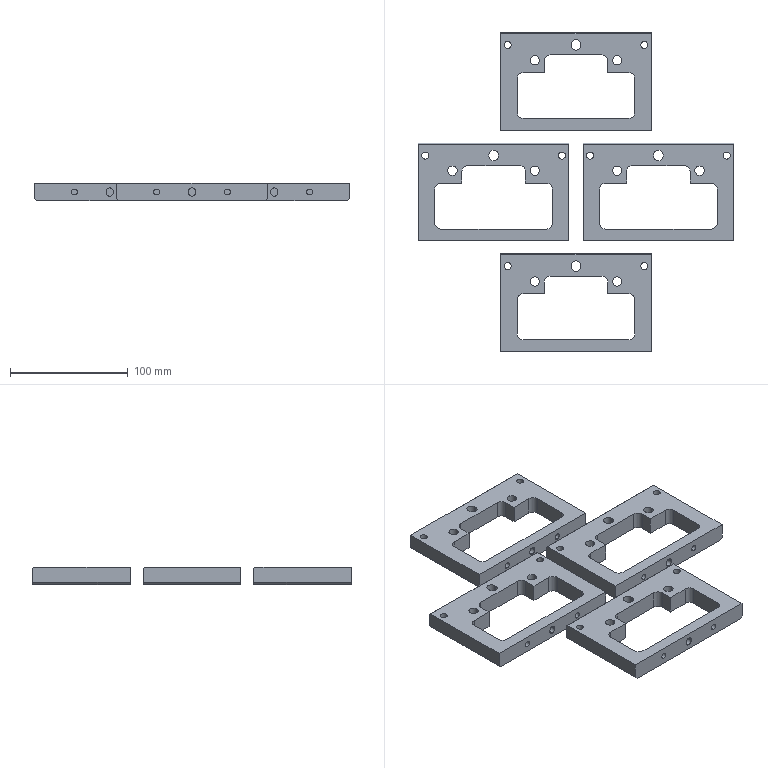NC program | NX | posted with a generic post | part box 268 x 271 x 15 mm
Lines 70 to 1437 of 34527:
(PLANAR_MILL , TOOL : D10)
N126 T10 M6
N128 G54
N130 G17 G0 G90 X-5.518 Y92.997 B0. C0. S9500 M3
N132 G43 Z30. H10
N134 Z0.7
N136 G94 G1 X-5.78 Y92.297 Z0.661 F1000.
N138 X-6.801 Y90.231 Z0.54
N140 X-8.022 Y88.277 Z0.419
N142 X-9.432 Y86.454 Z0.299
N144 X-10.243 Y85.6 Z0.237
N146 X0. Z-0.3
N148 X10.243 F3000.
N150 G2 X5.367 Y93.4 R23.1
N152 G1 X-5.367
N154 G2 X-10.243 Y85.6 R23.1
N156 G1 X0.
N158 Y79.6
N160 X32.9
N162 Y84.4
N164 X27.
N166 G2 X10.029 Y99.4 R17.1
N168 G1 X-10.029
N170 G2 X-27. Y84.4 R17.1
N172 G1 X-32.9
N174 Y79.6
N176 X0.
N178 Y73.6
N180 X38.9
N182 Y90.4
N184 X27.
N186 G2 X15.9 Y101.5 R11.1
N188 G1 Y105.4
N190 X-15.9
N192 Y101.5
N194 G2 X-27. Y90.4 R11.1
N196 G1 X-38.9
N198 Y73.6
N200 X0.
N202 Y67.6
N204 X44.9
N206 Y96.4
N208 X27.
N210 G2 X21.9 Y101.5 R5.1
N212 G1 Y111.4
N214 X-21.9
N216 Y101.5
N218 G2 X-27. Y96.4 R5.1
N220 G1 X-44.9
N222 Y67.6
N224 X0.
N226 Z0.4
N228 G0 X-5.518 Y92.997
N230 G1 X-5.78 Y92.297 Z0.361 F1000.
N232 X-6.801 Y90.231 Z0.24
N234 X-8.022 Y88.277 Z0.119
N236 X-9.432 Y86.454 Z-0.001
N238 X-10.243 Y85.6 Z-0.063
N240 X0. Z-0.6
N242 X10.243 F3000.
N244 G2 X5.367 Y93.4 R23.1
N246 G1 X-5.367
N248 G2 X-10.243 Y85.6 R23.1
N250 G1 X0.
N252 Y79.6
N254 X32.9
N256 Y84.4
N258 X27.
N260 G2 X10.029 Y99.4 R17.1
N262 G1 X-10.029
N264 G2 X-27. Y84.4 R17.1
N266 G1 X-32.9
N268 Y79.6
N270 X0.
N272 Y73.6
N274 X38.9
N276 Y90.4
N278 X27.
N280 G2 X15.9 Y101.5 R11.1
N282 G1 Y105.4
N284 X-15.9
N286 Y101.5
N288 G2 X-27. Y90.4 R11.1
N290 G1 X-38.9
N292 Y73.6
N294 X0.
N296 Y67.6
N298 X44.9
N300 Y96.4
N302 X27.
N304 G2 X21.9 Y101.5 R5.1
N306 G1 Y111.4
N308 X-21.9
N310 Y101.5
N312 G2 X-27. Y96.4 R5.1
N314 G1 X-44.9
N316 Y67.6
N318 X0.
N320 Z0.1
N322 G0 X-5.518 Y92.997
N324 G1 X-5.78 Y92.297 Z0.061 F1000.
N326 X-6.801 Y90.231 Z-0.06
N328 X-8.022 Y88.277 Z-0.181
N330 X-9.432 Y86.454 Z-0.301
N332 X-10.243 Y85.6 Z-0.363
N334 X0. Z-0.9
N336 X10.243 F3000.
N338 G2 X5.367 Y93.4 R23.1
N340 G1 X-5.367
N342 G2 X-10.243 Y85.6 R23.1
N344 G1 X0.
N346 Y79.6
N348 X32.9
N350 Y84.4
N352 X27.
N354 G2 X10.029 Y99.4 R17.1
N356 G1 X-10.029
N358 G2 X-27. Y84.4 R17.1
N360 G1 X-32.9
N362 Y79.6
N364 X0.
N366 Y73.6
N368 X38.9
N370 Y90.4
N372 X27.
N374 G2 X15.9 Y101.5 R11.1
N376 G1 Y105.4
N378 X-15.9
N380 Y101.5
N382 G2 X-27. Y90.4 R11.1
N384 G1 X-38.9
N386 Y73.6
N388 X0.
N390 Y67.6
N392 X44.9
N394 Y96.4
N396 X27.
N398 G2 X21.9 Y101.5 R5.1
N400 G1 Y111.4
N402 X-21.9
N404 Y101.5
N406 G2 X-27. Y96.4 R5.1
N408 G1 X-44.9
N410 Y67.6
N412 X0.
N414 Z-0.2
N416 G0 X-5.518 Y92.997
N418 G1 X-5.78 Y92.297 Z-0.239 F1000.
N420 X-6.801 Y90.231 Z-0.36
N422 X-8.022 Y88.277 Z-0.481
N424 X-9.432 Y86.454 Z-0.601
N426 X-10.243 Y85.6 Z-0.663
N428 X0. Z-1.2
N430 X10.243 F3000.
N432 G2 X5.367 Y93.4 R23.1
N434 G1 X-5.367
N436 G2 X-10.243 Y85.6 R23.1
N438 G1 X0.
N440 Y79.6
N442 X32.9
N444 Y84.4
N446 X27.
N448 G2 X10.029 Y99.4 R17.1
N450 G1 X-10.029
N452 G2 X-27. Y84.4 R17.1
N454 G1 X-32.9
N456 Y79.6
N458 X0.
N460 Y73.6
N462 X38.9
N464 Y90.4
N466 X27.
N468 G2 X15.9 Y101.5 R11.1
N470 G1 Y105.4
N472 X-15.9
N474 Y101.5
N476 G2 X-27. Y90.4 R11.1
N478 G1 X-38.9
N480 Y73.6
N482 X0.
N484 Y67.6
N486 X44.9
N488 Y96.4
N490 X27.
N492 G2 X21.9 Y101.5 R5.1
N494 G1 Y111.4
N496 X-21.9
N498 Y101.5
N500 G2 X-27. Y96.4 R5.1
N502 G1 X-44.9
N504 Y67.6
N506 X0.
N508 Z-0.5
N510 G0 X-5.518 Y92.997
N512 G1 X-5.78 Y92.297 Z-0.539 F1000.
N514 X-6.801 Y90.231 Z-0.66
N516 X-8.022 Y88.277 Z-0.781
N518 X-9.432 Y86.454 Z-0.901
N520 X-10.243 Y85.6 Z-0.963
N522 X0. Z-1.5
N524 X10.243 F3000.
N526 G2 X5.367 Y93.4 R23.1
N528 G1 X-5.367
N530 G2 X-10.243 Y85.6 R23.1
N532 G1 X0.
N534 Y79.6
N536 X32.9
N538 Y84.4
N540 X27.
N542 G2 X10.029 Y99.4 R17.1
N544 G1 X-10.029
N546 G2 X-27. Y84.4 R17.1
N548 G1 X-32.9
N550 Y79.6
N552 X0.
N554 Y73.6
N556 X38.9
N558 Y90.4
N560 X27.
N562 G2 X15.9 Y101.5 R11.1
N564 G1 Y105.4
N566 X-15.9
N568 Y101.5
N570 G2 X-27. Y90.4 R11.1
N572 G1 X-38.9
N574 Y73.6
N576 X0.
N578 Y67.6
N580 X44.9
N582 Y96.4
N584 X27.
N586 G2 X21.9 Y101.5 R5.1
N588 G1 Y111.4
N590 X-21.9
N592 Y101.5
N594 G2 X-27. Y96.4 R5.1
N596 G1 X-44.9
N598 Y67.6
N600 X0.
N602 Z-0.8
N604 G0 X-5.518 Y92.997
N606 G1 X-5.78 Y92.297 Z-0.839 F1000.
N608 X-6.801 Y90.231 Z-0.96
N610 X-8.022 Y88.277 Z-1.081
N612 X-9.432 Y86.454 Z-1.201
N614 X-10.243 Y85.6 Z-1.263
N616 X0. Z-1.8
N618 X10.243 F3000.
N620 G2 X5.367 Y93.4 R23.1
N622 G1 X-5.367
N624 G2 X-10.243 Y85.6 R23.1
N626 G1 X0.
N628 Y79.6
N630 X32.9
N632 Y84.4
N634 X27.
N636 G2 X10.029 Y99.4 R17.1
N638 G1 X-10.029
N640 G2 X-27. Y84.4 R17.1
N642 G1 X-32.9
N644 Y79.6
N646 X0.
N648 Y73.6
N650 X38.9
N652 Y90.4
N654 X27.
N656 G2 X15.9 Y101.5 R11.1
N658 G1 Y105.4
N660 X-15.9
N662 Y101.5
N664 G2 X-27. Y90.4 R11.1
N666 G1 X-38.9
N668 Y73.6
N670 X0.
N672 Y67.6
N674 X44.9
N676 Y96.4
N678 X27.
N680 G2 X21.9 Y101.5 R5.1
N682 G1 Y111.4
N684 X-21.9
N686 Y101.5
N688 G2 X-27. Y96.4 R5.1
N690 G1 X-44.9
N692 Y67.6
N694 X0.
N696 Z-1.1
N698 G0 X-5.518 Y92.997
N700 G1 X-5.78 Y92.297 Z-1.139 F1000.
N702 X-6.801 Y90.231 Z-1.26
N704 X-8.022 Y88.277 Z-1.381
N706 X-9.432 Y86.454 Z-1.501
N708 X-10.243 Y85.6 Z-1.563
N710 X0. Z-2.1
N712 X10.243 F3000.
N714 G2 X5.367 Y93.4 R23.1
N716 G1 X-5.367
N718 G2 X-10.243 Y85.6 R23.1
N720 G1 X0.
N722 Y79.6
N724 X32.9
N726 Y84.4
N728 X27.
N730 G2 X10.029 Y99.4 R17.1
N732 G1 X-10.029
N734 G2 X-27. Y84.4 R17.1
N736 G1 X-32.9
N738 Y79.6
N740 X0.
N742 Y73.6
N744 X38.9
N746 Y90.4
N748 X27.
N750 G2 X15.9 Y101.5 R11.1
N752 G1 Y105.4
N754 X-15.9
N756 Y101.5
N758 G2 X-27. Y90.4 R11.1
N760 G1 X-38.9
N762 Y73.6
N764 X0.
N766 Y67.6
N768 X44.9
N770 Y96.4
N772 X27.
N774 G2 X21.9 Y101.5 R5.1
N776 G1 Y111.4
N778 X-21.9
N780 Y101.5
N782 G2 X-27. Y96.4 R5.1
N784 G1 X-44.9
N786 Y67.6
N788 X0.
N790 Z-1.4
N792 G0 X-5.518 Y92.997
N794 G1 X-5.78 Y92.297 Z-1.439 F1000.
N796 X-6.801 Y90.231 Z-1.56
N798 X-8.022 Y88.277 Z-1.681
N800 X-9.432 Y86.454 Z-1.801
N802 X-10.243 Y85.6 Z-1.863
N804 X0. Z-2.4
N806 X10.243 F3000.
N808 G2 X5.367 Y93.4 R23.1
N810 G1 X-5.367
N812 G2 X-10.243 Y85.6 R23.1
N814 G1 X0.
N816 Y79.6
N818 X32.9
N820 Y84.4
N822 X27.
N824 G2 X10.029 Y99.4 R17.1
N826 G1 X-10.029
N828 G2 X-27. Y84.4 R17.1
N830 G1 X-32.9
N832 Y79.6
N834 X0.
N836 Y73.6
N838 X38.9
N840 Y90.4
N842 X27.
N844 G2 X15.9 Y101.5 R11.1
N846 G1 Y105.4
N848 X-15.9
N850 Y101.5
N852 G2 X-27. Y90.4 R11.1
N854 G1 X-38.9
N856 Y73.6
N858 X0.
N860 Y67.6
N862 X44.9
N864 Y96.4
N866 X27.
N868 G2 X21.9 Y101.5 R5.1
N870 G1 Y111.4
N872 X-21.9
N874 Y101.5
N876 G2 X-27. Y96.4 R5.1
N878 G1 X-44.9
N880 Y67.6
N882 X0.
N884 Z-1.7
N886 G0 X-5.518 Y92.997
N888 G1 X-5.78 Y92.297 Z-1.739 F1000.
N890 X-6.801 Y90.231 Z-1.86
N892 X-8.022 Y88.277 Z-1.981
N894 X-9.432 Y86.454 Z-2.101
N896 X-10.243 Y85.6 Z-2.163
N898 X0. Z-2.7
N900 X10.243 F3000.
N902 G2 X5.367 Y93.4 R23.1
N904 G1 X-5.367
N906 G2 X-10.243 Y85.6 R23.1
N908 G1 X0.
N910 Y79.6
N912 X32.9
N914 Y84.4
N916 X27.
N918 G2 X10.029 Y99.4 R17.1
N920 G1 X-10.029
N922 G2 X-27. Y84.4 R17.1
N924 G1 X-32.9
N926 Y79.6
N928 X0.
N930 Y73.6
N932 X38.9
N934 Y90.4
N936 X27.
N938 G2 X15.9 Y101.5 R11.1
N940 G1 Y105.4
N942 X-15.9
N944 Y101.5
N946 G2 X-27. Y90.4 R11.1
N948 G1 X-38.9
N950 Y73.6
N952 X0.
N954 Y67.6
N956 X44.9
N958 Y96.4
N960 X27.
N962 G2 X21.9 Y101.5 R5.1
N964 G1 Y111.4
N966 X-21.9
N968 Y101.5
N970 G2 X-27. Y96.4 R5.1
N972 G1 X-44.9
N974 Y67.6
N976 X0.
N978 Z-2.
N980 G0 X-5.518 Y92.997
N982 G1 X-5.78 Y92.297 Z-2.039 F1000.
N984 X-6.801 Y90.231 Z-2.16
N986 X-8.022 Y88.277 Z-2.281
N988 X-9.432 Y86.454 Z-2.401
N990 X-10.243 Y85.6 Z-2.463
N992 X0. Z-3.
N994 X10.243 F3000.
N996 G2 X5.367 Y93.4 R23.1
N998 G1 X-5.367
N1000 G2 X-10.243 Y85.6 R23.1
N1002 G1 X0.
N1004 Y79.6
N1006 X32.9
N1008 Y84.4
N1010 X27.
N1012 G2 X10.029 Y99.4 R17.1
N1014 G1 X-10.029
N1016 G2 X-27. Y84.4 R17.1
N1018 G1 X-32.9
N1020 Y79.6
N1022 X0.
N1024 Y73.6
N1026 X38.9
N1028 Y90.4
N1030 X27.
N1032 G2 X15.9 Y101.5 R11.1
N1034 G1 Y105.4
N1036 X-15.9
N1038 Y101.5
N1040 G2 X-27. Y90.4 R11.1
N1042 G1 X-38.9
N1044 Y73.6
N1046 X0.
N1048 Y67.6
N1050 X44.9
N1052 Y96.4
N1054 X27.
N1056 G2 X21.9 Y101.5 R5.1
N1058 G1 Y111.4
N1060 X-21.9
N1062 Y101.5
N1064 G2 X-27. Y96.4 R5.1
N1066 G1 X-44.9
N1068 Y67.6
N1070 X0.
N1072 Z-2.3
N1074 G0 X-5.518 Y92.997
N1076 G1 X-5.78 Y92.297 Z-2.339 F1000.
N1078 X-6.801 Y90.231 Z-2.46
N1080 X-8.022 Y88.277 Z-2.581
N1082 X-9.432 Y86.454 Z-2.701
N1084 X-10.243 Y85.6 Z-2.763
N1086 X0. Z-3.3
N1088 X10.243 F3000.
N1090 G2 X5.367 Y93.4 R23.1
N1092 G1 X-5.367
N1094 G2 X-10.243 Y85.6 R23.1
N1096 G1 X0.
N1098 Y79.6
N1100 X32.9
N1102 Y84.4
N1104 X27.
N1106 G2 X10.029 Y99.4 R17.1
N1108 G1 X-10.029
N1110 G2 X-27. Y84.4 R17.1
N1112 G1 X-32.9
N1114 Y79.6
N1116 X0.
N1118 Y73.6
N1120 X38.9
N1122 Y90.4
N1124 X27.
N1126 G2 X15.9 Y101.5 R11.1
N1128 G1 Y105.4
N1130 X-15.9
N1132 Y101.5
N1134 G2 X-27. Y90.4 R11.1
N1136 G1 X-38.9
N1138 Y73.6
N1140 X0.
N1142 Y67.6
N1144 X44.9
N1146 Y96.4
N1148 X27.
N1150 G2 X21.9 Y101.5 R5.1
N1152 G1 Y111.4
N1154 X-21.9
N1156 Y101.5
N1158 G2 X-27. Y96.4 R5.1
N1160 G1 X-44.9
N1162 Y67.6
N1164 X0.
N1166 Z-2.6
N1168 G0 X-5.518 Y92.997
N1170 G1 X-5.78 Y92.297 Z-2.639 F1000.
N1172 X-6.801 Y90.231 Z-2.76
N1174 X-8.022 Y88.277 Z-2.881
N1176 X-9.432 Y86.454 Z-3.001
N1178 X-10.243 Y85.6 Z-3.063
N1180 X0. Z-3.6
N1182 X10.243 F3000.
N1184 G2 X5.367 Y93.4 R23.1
N1186 G1 X-5.367
N1188 G2 X-10.243 Y85.6 R23.1
N1190 G1 X0.
N1192 Y79.6
N1194 X32.9
N1196 Y84.4
N1198 X27.
N1200 G2 X10.029 Y99.4 R17.1
N1202 G1 X-10.029
N1204 G2 X-27. Y84.4 R17.1
N1206 G1 X-32.9
N1208 Y79.6
N1210 X0.
N1212 Y73.6
N1214 X38.9
N1216 Y90.4
N1218 X27.
N1220 G2 X15.9 Y101.5 R11.1
N1222 G1 Y105.4
N1224 X-15.9
N1226 Y101.5
N1228 G2 X-27. Y90.4 R11.1
N1230 G1 X-38.9
N1232 Y73.6
N1234 X0.
N1236 Y67.6
N1238 X44.9
N1240 Y96.4
N1242 X27.
N1244 G2 X21.9 Y101.5 R5.1
N1246 G1 Y111.4
N1248 X-21.9
N1250 Y101.5
N1252 G2 X-27. Y96.4 R5.1
N1254 G1 X-44.9
N1256 Y67.6
N1258 X0.
N1260 Z-2.9
N1262 G0 X-5.518 Y92.997
N1264 G1 X-5.78 Y92.297 Z-2.939 F1000.
N1266 X-6.801 Y90.231 Z-3.06
N1268 X-8.022 Y88.277 Z-3.181
N1270 X-9.432 Y86.454 Z-3.301
N1272 X-10.243 Y85.6 Z-3.363
N1274 X0. Z-3.9
N1276 X10.243 F3000.
N1278 G2 X5.367 Y93.4 R23.1
N1280 G1 X-5.367
N1282 G2 X-10.243 Y85.6 R23.1
N1284 G1 X0.
N1286 Y79.6
N1288 X32.9
N1290 Y84.4
N1292 X27.
N1294 G2 X10.029 Y99.4 R17.1
N1296 G1 X-10.029
N1298 G2 X-27. Y84.4 R17.1
N1300 G1 X-32.9
N1302 Y79.6
N1304 X0.
N1306 Y73.6
N1308 X38.9
N1310 Y90.4
N1312 X27.
N1314 G2 X15.9 Y101.5 R11.1
N1316 G1 Y105.4
N1318 X-15.9
N1320 Y101.5
N1322 G2 X-27. Y90.4 R11.1
N1324 G1 X-38.9
N1326 Y73.6
N1328 X0.
N1330 Y67.6
N1332 X44.9
N1334 Y96.4
N1336 X27.
N1338 G2 X21.9 Y101.5 R5.1
N1340 G1 Y111.4
N1342 X-21.9
N1344 Y101.5
N1346 G2 X-27. Y96.4 R5.1
N1348 G1 X-44.9
N1350 Y67.6
N1352 X0.
N1354 Z-3.2
N1356 G0 X-5.518 Y92.997
N1358 G1 X-5.78 Y92.297 Z-3.239 F1000.
N1360 X-6.801 Y90.231 Z-3.36
N1362 X-8.022 Y88.277 Z-3.481
N1364 X-9.432 Y86.454 Z-3.601
N1366 X-10.243 Y85.6 Z-3.663
N1368 X0. Z-4.2
N1370 X10.243 F3000.
N1372 G2 X5.367 Y93.4 R23.1
N1374 G1 X-5.367
N1376 G2 X-10.243 Y85.6 R23.1
N1378 G1 X0.
N1380 Y79.6
N1382 X32.9
N1384 Y84.4
N1386 X27.
N1388 G2 X10.029 Y99.4 R17.1
N1390 G1 X-10.029
N1392 G2 X-27. Y84.4 R17.1
N1394 G1 X-32.9
N1396 Y79.6
N1398 X0.
N1400 Y73.6
N1402 X38.9
N1404 Y90.4
N1406 X27.
N1408 G2 X15.9 Y101.5 R11.1
N1410 G1 Y105.4
N1412 X-15.9
N1414 Y101.5
N1416 G2 X-27. Y90.4 R11.1
N1418 G1 X-38.9
N1420 Y73.6
N1422 X0.
N1424 Y67.6
N1426 X44.9
N1428 Y96.4
N1430 X27.
N1432 G2 X21.9 Y101.5 R5.1
N1434 G1 Y111.4
N1436 X-21.9
N1438 Y101.5
N1440 G2 X-27. Y96.4 R5.1
N1442 G1 X-44.9
N1444 Y67.6
N1446 X0.
N1448 Z-3.5
N1450 G0 X-5.518 Y92.997
N1452 G1 X-5.78 Y92.297 Z-3.539 F1000.
N1454 X-6.801 Y90.231 Z-3.66
N1456 X-8.022 Y88.277 Z-3.781
N1458 X-9.432 Y86.454 Z-3.901
N1460 X-10.243 Y85.6 Z-3.963
N1462 X0. Z-4.5
N1464 X10.243 F3000.
N1466 G2 X5.367 Y93.4 R23.1
N1468 G1 X-5.367
N1470 G2 X-10.243 Y85.6 R23.1
N1472 G1 X0.
N1474 Y79.6
N1476 X32.9
N1478 Y84.4
N1480 X27.
N1482 G2 X10.029 Y99.4 R17.1
N1484 G1 X-10.029
N1486 G2 X-27. Y84.4 R17.1
N1488 G1 X-32.9
N1490 Y79.6
N1492 X0.
N1494 Y73.6
N1496 X38.9
N1498 Y90.4
N1500 X27.
N1502 G2 X15.9 Y101.5 R11.1
N1504 G1 Y105.4
N1506 X-15.9
N1508 Y101.5
N1510 G2 X-27. Y90.4 R11.1
N1512 G1 X-38.9
N1514 Y73.6
N1516 X0.
N1518 Y67.6
N1520 X44.9
N1522 Y96.4
N1524 X27.
N1526 G2 X21.9 Y101.5 R5.1
N1528 G1 Y111.4
N1530 X-21.9
N1532 Y101.5
N1534 G2 X-27. Y96.4 R5.1
N1536 G1 X-44.9
N1538 Y67.6
N1540 X0.
N1542 Z-3.8
N1544 G0 X-5.518 Y92.997
N1546 G1 X-5.78 Y92.297 Z-3.839 F1000.
N1548 X-6.801 Y90.231 Z-3.96
N1550 X-8.022 Y88.277 Z-4.081
N1552 X-9.432 Y86.454 Z-4.201
N1554 X-10.243 Y85.6 Z-4.263
N1556 X0. Z-4.8
N1558 X10.243 F3000.
N1560 G2 X5.367 Y93.4 R23.1
N1562 G1 X-5.367
N1564 G2 X-10.243 Y85.6 R23.1
N1566 G1 X0.
N1568 Y79.6
N1570 X32.9
N1572 Y84.4
N1574 X27.
N1576 G2 X10.029 Y99.4 R17.1
N1578 G1 X-10.029
N1580 G2 X-27. Y84.4 R17.1
N1582 G1 X-32.9
N1584 Y79.6
N1586 X0.
N1588 Y73.6
N1590 X38.9
N1592 Y90.4
N1594 X27.
N1596 G2 X15.9 Y101.5 R11.1
N1598 G1 Y105.4
N1600 X-15.9
N1602 Y101.5
N1604 G2 X-27. Y90.4 R11.1
N1606 G1 X-38.9
N1608 Y73.6
N1610 X0.
N1612 Y67.6
N1614 X44.9
N1616 Y96.4
N1618 X27.
N1620 G2 X21.9 Y101.5 R5.1
N1622 G1 Y111.4
N1624 X-21.9
N1626 Y101.5
N1628 G2 X-27. Y96.4 R5.1
N1630 G1 X-44.9
N1632 Y67.6
N1634 X0.
N1636 Z-4.1
N1638 G0 X-5.518 Y92.997
N1640 G1 X-5.78 Y92.297 Z-4.139 F1000.
N1642 X-6.801 Y90.231 Z-4.26
N1644 X-8.022 Y88.277 Z-4.381
N1646 X-9.432 Y86.454 Z-4.501
N1648 X-10.243 Y85.6 Z-4.563
N1650 X0. Z-5.1
N1652 X10.243 F3000.
N1654 G2 X5.367 Y93.4 R23.1
N1656 G1 X-5.367
N1658 G2 X-10.243 Y85.6 R23.1
N1660 G1 X0.
N1662 Y79.6
N1664 X32.9
N1666 Y84.4
N1668 X27.
N1670 G2 X10.029 Y99.4 R17.1
N1672 G1 X-10.029
N1674 G2 X-27. Y84.4 R17.1
N1676 G1 X-32.9
N1678 Y79.6
N1680 X0.
N1682 Y73.6
N1684 X38.9
N1686 Y90.4
N1688 X27.
N1690 G2 X15.9 Y101.5 R11.1
N1692 G1 Y105.4
N1694 X-15.9
N1696 Y101.5
N1698 G2 X-27. Y90.4 R11.1
N1700 G1 X-38.9
N1702 Y73.6
N1704 X0.
N1706 Y67.6
N1708 X44.9
N1710 Y96.4
N1712 X27.
N1714 G2 X21.9 Y101.5 R5.1
N1716 G1 Y111.4
N1718 X-21.9
N1720 Y101.5
N1722 G2 X-27. Y96.4 R5.1
N1724 G1 X-44.9
N1726 Y67.6
N1728 X0.
N1730 Z-4.4
N1732 G0 X-5.518 Y92.997
N1734 G1 X-5.78 Y92.297 Z-4.439 F1000.
N1736 X-6.801 Y90.231 Z-4.56
N1738 X-8.022 Y88.277 Z-4.681
N1740 X-9.432 Y86.454 Z-4.801
N1742 X-10.243 Y85.6 Z-4.863
N1744 X0. Z-5.4
N1746 X10.243 F3000.
N1748 G2 X5.367 Y93.4 R23.1
N1750 G1 X-5.367
N1752 G2 X-10.243 Y85.6 R23.1
N1754 G1 X0.
N1756 Y79.6
N1758 X32.9
N1760 Y84.4
N1762 X27.
N1764 G2 X10.029 Y99.4 R17.1
N1766 G1 X-10.029
N1768 G2 X-27. Y84.4 R17.1
N1770 G1 X-32.9
N1772 Y79.6
N1774 X0.
N1776 Y73.6
N1778 X38.9
N1780 Y90.4
N1782 X27.
N1784 G2 X15.9 Y101.5 R11.1
N1786 G1 Y105.4
N1788 X-15.9
N1790 Y101.5
N1792 G2 X-27. Y90.4 R11.1
N1794 G1 X-38.9
N1796 Y73.6
N1798 X0.
N1800 Y67.6
N1802 X44.9
N1804 Y96.4
N1806 X27.
N1808 G2 X21.9 Y101.5 R5.1
N1810 G1 Y111.4
N1812 X-21.9
N1814 Y101.5
N1816 G2 X-27. Y96.4 R5.1
N1818 G1 X-44.9
N1820 Y67.6
N1822 X0.
N1824 Z-4.7
N1826 G0 X-5.518 Y92.997
N1828 G1 X-5.78 Y92.297 Z-4.739 F1000.
N1830 X-6.801 Y90.231 Z-4.86
N1832 X-8.022 Y88.277 Z-4.981
N1834 X-9.432 Y86.454 Z-5.101
N1836 X-10.243 Y85.6 Z-5.163
N1838 X0. Z-5.7
N1840 X10.243 F3000.
N1842 G2 X5.367 Y93.4 R23.1
N1844 G1 X-5.367
N1846 G2 X-10.243 Y85.6 R23.1
N1848 G1 X0.
N1850 Y79.6
N1852 X32.9
N1854 Y84.4
N1856 X27.
N1858 G2 X10.029 Y99.4 R17.1
N1860 G1 X-10.029
N1862 G2 X-27. Y84.4 R17.1
N1864 G1 X-32.9
N1866 Y79.6
N1868 X0.
N1870 Y73.6
N1872 X38.9
N1874 Y90.4
N1876 X27.
N1878 G2 X15.9 Y101.5 R11.1
N1880 G1 Y105.4
N1882 X-15.9
N1884 Y101.5
N1886 G2 X-27. Y90.4 R11.1
N1888 G1 X-38.9
N1890 Y73.6
N1892 X0.
N1894 Y67.6
N1896 X44.9
N1898 Y96.4
N1900 X27.
N1902 G2 X21.9 Y101.5 R5.1
N1904 G1 Y111.4
N1906 X-21.9
N1908 Y101.5
N1910 G2 X-27. Y96.4 R5.1
N1912 G1 X-44.9
N1914 Y67.6
N1916 X0.
N1918 Z-5.
N1920 G0 X-5.518 Y92.997
N1922 G1 X-5.78 Y92.297 Z-5.039 F1000.
N1924 X-6.801 Y90.231 Z-5.16
N1926 X-8.022 Y88.277 Z-5.281
N1928 X-9.432 Y86.454 Z-5.401
N1930 X-10.243 Y85.6 Z-5.463
N1932 X0. Z-6.
N1934 X10.243 F3000.
N1936 G2 X5.367 Y93.4 R23.1
N1938 G1 X-5.367
N1940 G2 X-10.243 Y85.6 R23.1
N1942 G1 X0.
N1944 Y79.6
N1946 X32.9
N1948 Y84.4
N1950 X27.
N1952 G2 X10.029 Y99.4 R17.1
N1954 G1 X-10.029
N1956 G2 X-27. Y84.4 R17.1
N1958 G1 X-32.9
N1960 Y79.6
N1962 X0.
N1964 Y73.6
N1966 X38.9
N1968 Y90.4
N1970 X27.
N1972 G2 X15.9 Y101.5 R11.1
N1974 G1 Y105.4
N1976 X-15.9
N1978 Y101.5
N1980 G2 X-27. Y90.4 R11.1
N1982 G1 X-38.9
N1984 Y73.6
N1986 X0.
N1988 Y67.6
N1990 X44.9
N1992 Y96.4
N1994 X27.
N1996 G2 X21.9 Y101.5 R5.1
N1998 G1 Y111.4
N2000 X-21.9
N2002 Y101.5
N2004 G2 X-27. Y96.4 R5.1
N2006 G1 X-44.9
N2008 Y67.6
N2010 X0.
N2012 Z-5.3
N2014 G0 X-5.518 Y92.997
N2016 G1 X-5.78 Y92.297 Z-5.339 F1000.
N2018 X-6.801 Y90.231 Z-5.46
N2020 X-8.022 Y88.277 Z-5.581
N2022 X-9.432 Y86.454 Z-5.701
N2024 X-10.243 Y85.6 Z-5.763
N2026 X0. Z-6.3
N2028 X10.243 F3000.
N2030 G2 X5.367 Y93.4 R23.1
N2032 G1 X-5.367
N2034 G2 X-10.243 Y85.6 R23.1
N2036 G1 X0.
N2038 Y79.6
N2040 X32.9
N2042 Y84.4
N2044 X27.
N2046 G2 X10.029 Y99.4 R17.1
N2048 G1 X-10.029
N2050 G2 X-27. Y84.4 R17.1
N2052 G1 X-32.9
N2054 Y79.6
N2056 X0.
N2058 Y73.6
N2060 X38.9
N2062 Y90.4
N2064 X27.
N2066 G2 X15.9 Y101.5 R11.1
N2068 G1 Y105.4
N2070 X-15.9
N2072 Y101.5
N2074 G2 X-27. Y90.4 R11.1
N2076 G1 X-38.9
N2078 Y73.6
N2080 X0.
N2082 Y67.6
N2084 X44.9
N2086 Y96.4
N2088 X27.
N2090 G2 X21.9 Y101.5 R5.1
N2092 G1 Y111.4
N2094 X-21.9
N2096 Y101.5
N2098 G2 X-27. Y96.4 R5.1
N2100 G1 X-44.9
N2102 Y67.6
N2104 X0.
N2106 Z-5.6
N2108 G0 X-5.518 Y92.997
N2110 G1 X-5.78 Y92.297 Z-5.639 F1000.
N2112 X-6.801 Y90.231 Z-5.76
N2114 X-8.022 Y88.277 Z-5.881
N2116 X-9.432 Y86.454 Z-6.001
N2118 X-10.243 Y85.6 Z-6.063
N2120 X0. Z-6.6
N2122 X10.243 F3000.
N2124 G2 X5.367 Y93.4 R23.1
N2126 G1 X-5.367
N2128 G2 X-10.243 Y85.6 R23.1
N2130 G1 X0.
N2132 Y79.6
N2134 X32.9
N2136 Y84.4
N2138 X27.
N2140 G2 X10.029 Y99.4 R17.1
N2142 G1 X-10.029
N2144 G2 X-27. Y84.4 R17.1
N2146 G1 X-32.9
N2148 Y79.6
N2150 X0.
N2152 Y73.6
N2154 X38.9
N2156 Y90.4
N2158 X27.
N2160 G2 X15.9 Y101.5 R11.1
N2162 G1 Y105.4
N2164 X-15.9
N2166 Y101.5
N2168 G2 X-27. Y90.4 R11.1
N2170 G1 X-38.9
N2172 Y73.6
N2174 X0.
N2176 Y67.6
N2178 X44.9
N2180 Y96.4
N2182 X27.
N2184 G2 X21.9 Y101.5 R5.1
N2186 G1 Y111.4
N2188 X-21.9
N2190 Y101.5
N2192 G2 X-27. Y96.4 R5.1
N2194 G1 X-44.9
N2196 Y67.6
N2198 X0.
N2200 Z-5.9
N2202 G0 X-5.518 Y92.997
N2204 G1 X-5.78 Y92.297 Z-5.939 F1000.
N2206 X-6.801 Y90.231 Z-6.06
N2208 X-8.022 Y88.277 Z-6.181
N2210 X-9.432 Y86.454 Z-6.301
N2212 X-10.243 Y85.6 Z-6.363
N2214 X0. Z-6.9
N2216 X10.243 F3000.
N2218 G2 X5.367 Y93.4 R23.1
N2220 G1 X-5.367
N2222 G2 X-10.243 Y85.6 R23.1
N2224 G1 X0.
N2226 Y79.6
N2228 X32.9
N2230 Y84.4
N2232 X27.
N2234 G2 X10.029 Y99.4 R17.1
N2236 G1 X-10.029
N2238 G2 X-27. Y84.4 R17.1
N2240 G1 X-32.9
N2242 Y79.6
N2244 X0.
N2246 Y73.6
N2248 X38.9
N2250 Y90.4
N2252 X27.
N2254 G2 X15.9 Y101.5 R11.1
N2256 G1 Y105.4
N2258 X-15.9
N2260 Y101.5
N2262 G2 X-27. Y90.4 R11.1
N2264 G1 X-38.9
N2266 Y73.6
N2268 X0.
N2270 Y67.6
N2272 X44.9
N2274 Y96.4
N2276 X27.
N2278 G2 X21.9 Y101.5 R5.1
N2280 G1 Y111.4
N2282 X-21.9
N2284 Y101.5
N2286 G2 X-27. Y96.4 R5.1
N2288 G1 X-44.9
N2290 Y67.6
N2292 X0.
N2294 Z-6.2
N2296 G0 X-5.518 Y92.997
N2298 G1 X-5.78 Y92.297 Z-6.239 F1000.
N2300 X-6.801 Y90.231 Z-6.36
N2302 X-8.022 Y88.277 Z-6.481
N2304 X-9.432 Y86.454 Z-6.601
N2306 X-10.243 Y85.6 Z-6.663
N2308 X0. Z-7.2
N2310 X10.243 F3000.
N2312 G2 X5.367 Y93.4 R23.1
N2314 G1 X-5.367
N2316 G2 X-10.243 Y85.6 R23.1
N2318 G1 X0.
N2320 Y79.6
N2322 X32.9
N2324 Y84.4
N2326 X27.
N2328 G2 X10.029 Y99.4 R17.1
N2330 G1 X-10.029
N2332 G2 X-27. Y84.4 R17.1
N2334 G1 X-32.9
N2336 Y79.6
N2338 X0.
N2340 Y73.6
N2342 X38.9
N2344 Y90.4
N2346 X27.
N2348 G2 X15.9 Y101.5 R11.1
N2350 G1 Y105.4
N2352 X-15.9
N2354 Y101.5
N2356 G2 X-27. Y90.4 R11.1
N2358 G1 X-38.9
N2360 Y73.6
N2362 X0.
N2364 Y67.6
N2366 X44.9
N2368 Y96.4
N2370 X27.
N2372 G2 X21.9 Y101.5 R5.1
N2374 G1 Y111.4
N2376 X-21.9
N2378 Y101.5
N2380 G2 X-27. Y96.4 R5.1
N2382 G1 X-44.9
N2384 Y67.6
N2386 X0.
N2388 Z-6.5
N2390 G0 X-5.518 Y92.997
N2392 G1 X-5.78 Y92.297 Z-6.539 F1000.
N2394 X-6.801 Y90.231 Z-6.66
N2396 X-8.022 Y88.277 Z-6.781
N2398 X-9.432 Y86.454 Z-6.901
N2400 X-10.243 Y85.6 Z-6.963
N2402 X0. Z-7.5
N2404 X10.243 F3000.
N2406 G2 X5.367 Y93.4 R23.1
N2408 G1 X-5.367
N2410 G2 X-10.243 Y85.6 R23.1
N2412 G1 X0.
N2414 Y79.6
N2416 X32.9
N2418 Y84.4
N2420 X27.
N2422 G2 X10.029 Y99.4 R17.1
N2424 G1 X-10.029
N2426 G2 X-27. Y84.4 R17.1
N2428 G1 X-32.9
N2430 Y79.6
N2432 X0.
N2434 Y73.6
N2436 X38.9
N2438 Y90.4
N2440 X27.
N2442 G2 X15.9 Y101.5 R11.1
N2444 G1 Y105.4
N2446 X-15.9
N2448 Y101.5
N2450 G2 X-27. Y90.4 R11.1
N2452 G1 X-38.9
N2454 Y73.6
N2456 X0.
N2458 Y67.6
N2460 X44.9
N2462 Y96.4
N2464 X27.
N2466 G2 X21.9 Y101.5 R5.1
N2468 G1 Y111.4
N2470 X-21.9
N2472 Y101.5
N2474 G2 X-27. Y96.4 R5.1
N2476 G1 X-44.9
N2478 Y67.6
N2480 X0.
N2482 Z-6.8
N2484 G0 X-5.518 Y92.997
N2486 G1 X-5.78 Y92.297 Z-6.839 F1000.
N2488 X-6.801 Y90.231 Z-6.96
N2490 X-8.022 Y88.277 Z-7.081
N2492 X-9.432 Y86.454 Z-7.201
N2494 X-10.243 Y85.6 Z-7.263
N2496 X0. Z-7.8
N2498 X10.243 F3000.
N2500 G2 X5.367 Y93.4 R23.1
N2502 G1 X-5.367
N2504 G2 X-10.243 Y85.6 R23.1
N2506 G1 X0.
N2508 Y79.6
N2510 X32.9
N2512 Y84.4
N2514 X27.
N2516 G2 X10.029 Y99.4 R17.1
N2518 G1 X-10.029
N2520 G2 X-27. Y84.4 R17.1
N2522 G1 X-32.9
N2524 Y79.6
N2526 X0.
N2528 Y73.6
N2530 X38.9
N2532 Y90.4
N2534 X27.
N2536 G2 X15.9 Y101.5 R11.1
N2538 G1 Y105.4
N2540 X-15.9
N2542 Y101.5
N2544 G2 X-27. Y90.4 R11.1
N2546 G1 X-38.9
N2548 Y73.6
N2550 X0.
N2552 Y67.6
N2554 X44.9
N2556 Y96.4
N2558 X27.
N2560 G2 X21.9 Y101.5 R5.1
N2562 G1 Y111.4
N2564 X-21.9
N2566 Y101.5
N2568 G2 X-27. Y96.4 R5.1
N2570 G1 X-44.9
N2572 Y67.6
N2574 X0.
N2576 Z-7.1
N2578 G0 X-5.518 Y92.997
N2580 G1 X-5.78 Y92.297 Z-7.139 F1000.
N2582 X-6.801 Y90.231 Z-7.26
N2584 X-8.022 Y88.277 Z-7.381
N2586 X-9.432 Y86.454 Z-7.501
N2588 X-10.243 Y85.6 Z-7.563
N2590 X0. Z-8.1
N2592 X10.243 F3000.
N2594 G2 X5.367 Y93.4 R23.1
N2596 G1 X-5.367
N2598 G2 X-10.243 Y85.6 R23.1
N2600 G1 X0.
N2602 Y79.6
N2604 X32.9
N2606 Y84.4
N2608 X27.
N2610 G2 X10.029 Y99.4 R17.1
N2612 G1 X-10.029
N2614 G2 X-27. Y84.4 R17.1
N2616 G1 X-32.9
N2618 Y79.6
N2620 X0.
N2622 Y73.6
N2624 X38.9
N2626 Y90.4
N2628 X27.
N2630 G2 X15.9 Y101.5 R11.1
N2632 G1 Y105.4
N2634 X-15.9
N2636 Y101.5
N2638 G2 X-27. Y90.4 R11.1
N2640 G1 X-38.9
N2642 Y73.6
N2644 X0.
N2646 Y67.6
N2648 X44.9
N2650 Y96.4
N2652 X27.
N2654 G2 X21.9 Y101.5 R5.1
N2656 G1 Y111.4
N2658 X-21.9
N2660 Y101.5
N2662 G2 X-27. Y96.4 R5.1
N2664 G1 X-44.9
N2666 Y67.6
N2668 X0.
N2670 Z-7.4
N2672 G0 X-5.518 Y92.997
N2674 G1 X-5.78 Y92.297 Z-7.439 F1000.
N2676 X-6.801 Y90.231 Z-7.56
N2678 X-8.022 Y88.277 Z-7.681
N2680 X-9.432 Y86.454 Z-7.801
N2682 X-10.243 Y85.6 Z-7.863
N2684 X0. Z-8.4
N2686 X10.243 F3000.
N2688 G2 X5.367 Y93.4 R23.1
N2690 G1 X-5.367
N2692 G2 X-10.243 Y85.6 R23.1
N2694 G1 X0.
N2696 Y79.6
N2698 X32.9
N2700 Y84.4
N2702 X27.
N2704 G2 X10.029 Y99.4 R17.1
N2706 G1 X-10.029
N2708 G2 X-27. Y84.4 R17.1
N2710 G1 X-32.9
N2712 Y79.6
N2714 X0.
N2716 Y73.6
N2718 X38.9
N2720 Y90.4
N2722 X27.
N2724 G2 X15.9 Y101.5 R11.1
N2726 G1 Y105.4
N2728 X-15.9
N2730 Y101.5
N2732 G2 X-27. Y90.4 R11.1
N2734 G1 X-38.9
N2736 Y73.6
N2738 X0.
N2740 Y67.6
N2742 X44.9
N2744 Y96.4
N2746 X27.
N2748 G2 X21.9 Y101.5 R5.1
N2750 G1 Y111.4
N2752 X-21.9
N2754 Y101.5
N2756 G2 X-27. Y96.4 R5.1
N2758 G1 X-44.9
N2760 Y67.6
N2762 X0.
N2764 Z-7.7
N2766 G0 X-5.518 Y92.997
N2768 G1 X-5.78 Y92.297 Z-7.739 F1000.
N2770 X-6.801 Y90.231 Z-7.86
N2772 X-8.022 Y88.277 Z-7.981
N2774 X-9.432 Y86.454 Z-8.101
N2776 X-10.243 Y85.6 Z-8.163
N2778 X0. Z-8.7
N2780 X10.243 F3000.
N2782 G2 X5.367 Y93.4 R23.1
N2784 G1 X-5.367
N2786 G2 X-10.243 Y85.6 R23.1
N2788 G1 X0.
N2790 Y79.6
N2792 X32.9
N2794 Y84.4
N2796 X27.
N2798 G2 X10.029 Y99.4 R17.1
N2800 G1 X-10.029
N2802 G2 X-27. Y84.4 R17.1
N2804 G1 X-32.9
N2806 Y79.6
N2808 X0.
N2810 Y73.6
N2812 X38.9
N2814 Y90.4
N2816 X27.
N2818 G2 X15.9 Y101.5 R11.1
N2820 G1 Y105.4
N2822 X-15.9
N2824 Y101.5
N2826 G2 X-27. Y90.4 R11.1
N2828 G1 X-38.9
N2830 Y73.6
N2832 X0.
N2834 Y67.6
N2836 X44.9
N2838 Y96.4
N2840 X27.
N2842 G2 X21.9 Y101.5 R5.1
N2844 G1 Y111.4
N2846 X-21.9
N2848 Y101.5
N2850 G2 X-27. Y96.4 R5.1
N2852 G1 X-44.9
N2854 Y67.6